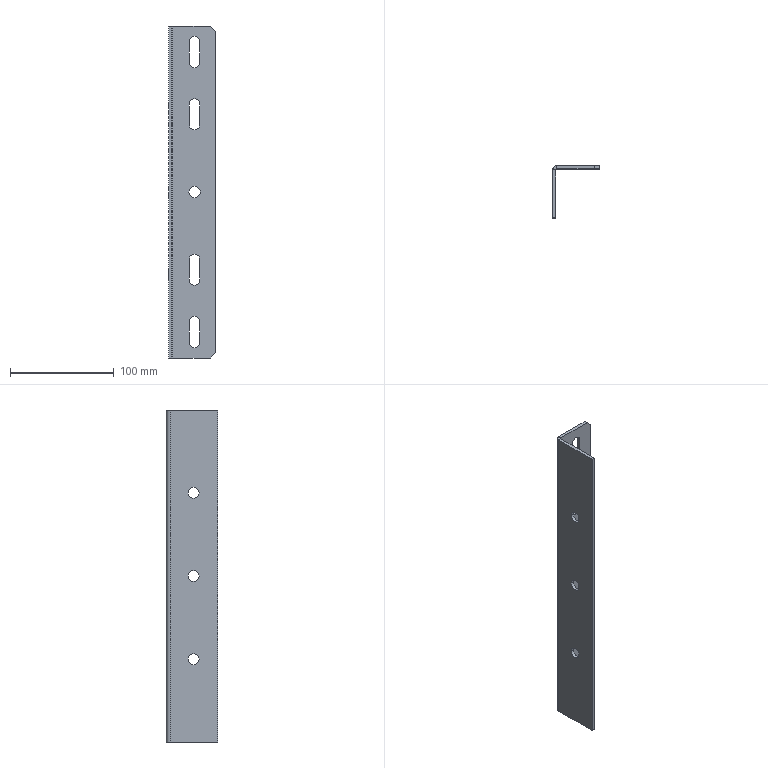Part | SolidWorks | features ICE 3, Chamfer 1, FlatPattern 1, SMBaseFlange 1, SheetMetal 1 | 1 solid | 40 faces | box 45 x 50 x 319.5 mm | volume 82672 mm3 | plane 22 | cylinder 18 | commonest cylinder face diameters 10 x8 10.5 x6 11 x2 2 x1 8 x1
STEP:
#1=CARTESIAN_POINT('',(30.5,0.,0.));
#2=VERTEX_POINT('',#1);
#3=CARTESIAN_POINT('',(19.5,0.,0.));
#4=VERTEX_POINT('',#3);
#5=CARTESIAN_POINT('',(25.,0.,0.));
#6=DIRECTION('',(0.,1.,0.));
#7=DIRECTION('',(1.,0.,0.));
#8=AXIS2_PLACEMENT_3D('',#5,#6,#7);
#9=CIRCLE('',#8,5.5);
#10=EDGE_CURVE('',#2,#4,#9,.T.);
#11=ORIENTED_EDGE('',*,*,#10,.T.);
#12=CARTESIAN_POINT('',(19.5,-3.,0.));
#13=VERTEX_POINT('',#12);
#14=CARTESIAN_POINT('',(19.5,0.000012,0.));
#15=DIRECTION('',(0.,-1.,0.));
#16=VECTOR('',#15,1000.);
#17=LINE('',#14,#16);
#18=EDGE_CURVE('',#4,#13,#17,.T.);
#19=ORIENTED_EDGE('',*,*,#18,.T.);
#20=CARTESIAN_POINT('',(30.5,-3.,0.));
#21=VERTEX_POINT('',#20);
#22=CARTESIAN_POINT('',(25.,-3.,0.));
#23=DIRECTION('',(0.,1.,0.));
#24=DIRECTION('',(1.,0.,0.));
#25=AXIS2_PLACEMENT_3D('',#22,#23,#24);
#26=CIRCLE('',#25,5.5);
#27=EDGE_CURVE('',#21,#13,#26,.T.);
#28=ORIENTED_EDGE('',*,*,#27,.F.);
#29=CARTESIAN_POINT('',(30.5,0.000012,0.));
#30=DIRECTION('',(0.,-1.,0.));
#31=VECTOR('',#30,1000.);
#32=LINE('',#29,#31);
#33=EDGE_CURVE('',#2,#21,#32,.T.);
#34=ORIENTED_EDGE('',*,*,#33,.F.);
#35=EDGE_LOOP('',(#11,#19,#28,#34));
#36=FACE_OUTER_BOUND('',#35,.T.);
#37=CARTESIAN_POINT('',(25.,0.000012,0.));
#38=DIRECTION('',(0.,-1.,0.));
#39=DIRECTION('',(1.,0.,0.));
#40=AXIS2_PLACEMENT_3D('',#37,#38,#39);
#41=CYLINDRICAL_SURFACE('',#40,5.5);
#42=ADVANCED_FACE('',(#36),#41,.F.);
#43=CARTESIAN_POINT('',(3.,-31.75,80.));
#44=VERTEX_POINT('',#43);
#45=CARTESIAN_POINT('',(3.,-21.25,80.));
#46=VERTEX_POINT('',#45);
#47=CARTESIAN_POINT('',(3.,-26.5,80.));
#48=DIRECTION('',(1.,0.,0.));
#49=DIRECTION('',(0.,1.,0.));
#50=AXIS2_PLACEMENT_3D('',#47,#48,#49);
#51=CIRCLE('',#50,5.25);
#52=EDGE_CURVE('',#44,#46,#51,.T.);
#53=ORIENTED_EDGE('',*,*,#52,.T.);
#54=CARTESIAN_POINT('',(0.,-21.25,80.));
#55=VERTEX_POINT('',#54);
#56=CARTESIAN_POINT('',(10.,-21.25,80.));
#57=DIRECTION('',(-1.,0.,0.));
#58=VECTOR('',#57,1000.);
#59=LINE('',#56,#58);
#60=EDGE_CURVE('',#46,#55,#59,.T.);
#61=ORIENTED_EDGE('',*,*,#60,.T.);
#62=CARTESIAN_POINT('',(0.,-31.75,80.));
#63=VERTEX_POINT('',#62);
#64=CARTESIAN_POINT('',(0.,-26.5,80.));
#65=DIRECTION('',(-1.,0.,0.));
#66=DIRECTION('',(0.,-1.,0.));
#67=AXIS2_PLACEMENT_3D('',#64,#65,#66);
#68=CIRCLE('',#67,5.25);
#69=EDGE_CURVE('',#55,#63,#68,.T.);
#70=ORIENTED_EDGE('',*,*,#69,.T.);
#71=CARTESIAN_POINT('',(10.,-31.75,80.));
#72=DIRECTION('',(-1.,0.,0.));
#73=VECTOR('',#72,1000.);
#74=LINE('',#71,#73);
#75=EDGE_CURVE('',#44,#63,#74,.T.);
#76=ORIENTED_EDGE('',*,*,#75,.F.);
#77=EDGE_LOOP('',(#53,#61,#70,#76));
#78=FACE_OUTER_BOUND('',#77,.T.);
#79=CARTESIAN_POINT('',(10.,-26.5,80.));
#80=DIRECTION('',(-1.,0.,0.));
#81=DIRECTION('',(0.,-1.,0.));
#82=AXIS2_PLACEMENT_3D('',#79,#80,#81);
#83=CYLINDRICAL_SURFACE('',#82,5.25);
#84=ADVANCED_FACE('',(#78),#83,.F.);
#85=CARTESIAN_POINT('',(3.,-31.75,0.));
#86=VERTEX_POINT('',#85);
#87=CARTESIAN_POINT('',(3.,-21.25,0.));
#88=VERTEX_POINT('',#87);
#89=CARTESIAN_POINT('',(3.,-26.5,0.));
#90=DIRECTION('',(1.,0.,0.));
#91=DIRECTION('',(0.,1.,0.));
#92=AXIS2_PLACEMENT_3D('',#89,#90,#91);
#93=CIRCLE('',#92,5.25);
#94=EDGE_CURVE('',#86,#88,#93,.T.);
#95=ORIENTED_EDGE('',*,*,#94,.T.);
#96=CARTESIAN_POINT('',(0.,-21.25,0.));
#97=VERTEX_POINT('',#96);
#98=CARTESIAN_POINT('',(10.,-21.25,0.));
#99=DIRECTION('',(-1.,0.,0.));
#100=VECTOR('',#99,1000.);
#101=LINE('',#98,#100);
#102=EDGE_CURVE('',#88,#97,#101,.T.);
#103=ORIENTED_EDGE('',*,*,#102,.T.);
#104=CARTESIAN_POINT('',(0.,-31.75,0.));
#105=VERTEX_POINT('',#104);
#106=CARTESIAN_POINT('',(0.,-26.5,0.));
#107=DIRECTION('',(-1.,0.,0.));
#108=DIRECTION('',(0.,-1.,0.));
#109=AXIS2_PLACEMENT_3D('',#106,#107,#108);
#110=CIRCLE('',#109,5.25);
#111=EDGE_CURVE('',#97,#105,#110,.T.);
#112=ORIENTED_EDGE('',*,*,#111,.T.);
#113=CARTESIAN_POINT('',(10.,-31.75,0.));
#114=DIRECTION('',(-1.,0.,0.));
#115=VECTOR('',#114,1000.);
#116=LINE('',#113,#115);
#117=EDGE_CURVE('',#86,#105,#116,.T.);
#118=ORIENTED_EDGE('',*,*,#117,.F.);
#119=EDGE_LOOP('',(#95,#103,#112,#118));
#120=FACE_OUTER_BOUND('',#119,.T.);
#121=CARTESIAN_POINT('',(10.,-26.5,0.));
#122=DIRECTION('',(-1.,0.,0.));
#123=DIRECTION('',(0.,-1.,0.));
#124=AXIS2_PLACEMENT_3D('',#121,#122,#123);
#125=CYLINDRICAL_SURFACE('',#124,5.25);
#126=ADVANCED_FACE('',(#120),#125,.F.);
#127=CARTESIAN_POINT('',(3.,-31.75,-80.));
#128=VERTEX_POINT('',#127);
#129=CARTESIAN_POINT('',(3.,-21.25,-80.));
#130=VERTEX_POINT('',#129);
#131=CARTESIAN_POINT('',(3.,-26.5,-80.));
#132=DIRECTION('',(1.,0.,0.));
#133=DIRECTION('',(0.,1.,0.));
#134=AXIS2_PLACEMENT_3D('',#131,#132,#133);
#135=CIRCLE('',#134,5.25);
#136=EDGE_CURVE('',#128,#130,#135,.T.);
#137=ORIENTED_EDGE('',*,*,#136,.T.);
#138=CARTESIAN_POINT('',(0.,-21.25,-80.));
#139=VERTEX_POINT('',#138);
#140=CARTESIAN_POINT('',(10.,-21.25,-80.));
#141=DIRECTION('',(-1.,0.,0.));
#142=VECTOR('',#141,1000.);
#143=LINE('',#140,#142);
#144=EDGE_CURVE('',#130,#139,#143,.T.);
#145=ORIENTED_EDGE('',*,*,#144,.T.);
#146=CARTESIAN_POINT('',(0.,-31.75,-80.));
#147=VERTEX_POINT('',#146);
#148=CARTESIAN_POINT('',(0.,-26.5,-80.));
#149=DIRECTION('',(-1.,0.,0.));
#150=DIRECTION('',(0.,-1.,0.));
#151=AXIS2_PLACEMENT_3D('',#148,#149,#150);
#152=CIRCLE('',#151,5.25);
#153=EDGE_CURVE('',#139,#147,#152,.T.);
#154=ORIENTED_EDGE('',*,*,#153,.T.);
#155=CARTESIAN_POINT('',(10.,-31.75,-80.));
#156=DIRECTION('',(-1.,0.,0.));
#157=VECTOR('',#156,1000.);
#158=LINE('',#155,#157);
#159=EDGE_CURVE('',#128,#147,#158,.T.);
#160=ORIENTED_EDGE('',*,*,#159,.F.);
#161=EDGE_LOOP('',(#137,#145,#154,#160));
#162=FACE_OUTER_BOUND('',#161,.T.);
#163=CARTESIAN_POINT('',(10.,-26.5,-80.));
#164=DIRECTION('',(-1.,0.,0.));
#165=DIRECTION('',(0.,-1.,0.));
#166=AXIS2_PLACEMENT_3D('',#163,#164,#165);
#167=CYLINDRICAL_SURFACE('',#166,5.25);
#168=ADVANCED_FACE('',(#162),#167,.F.);
#169=CARTESIAN_POINT('',(4.,0.,159.75));
#170=VERTEX_POINT('',#169);
#171=CARTESIAN_POINT('',(4.,-3.,159.75));
#172=VERTEX_POINT('',#171);
#173=CARTESIAN_POINT('',(4.,0.,159.75));
#174=DIRECTION('',(0.,-1.,0.));
#175=VECTOR('',#174,1000.);
#176=LINE('',#173,#175);
#177=EDGE_CURVE('',#170,#172,#176,.T.);
#178=ORIENTED_EDGE('',*,*,#177,.F.);
#179=CARTESIAN_POINT('',(0.,-4.,159.75));
#180=VERTEX_POINT('',#179);
#181=CARTESIAN_POINT('',(4.,-4.,159.75));
#182=DIRECTION('',(0.,0.,1.));
#183=DIRECTION('',(-1.,0.,0.));
#184=AXIS2_PLACEMENT_3D('',#181,#182,#183);
#185=CIRCLE('',#184,4.);
#186=EDGE_CURVE('',#170,#180,#185,.T.);
#187=ORIENTED_EDGE('',*,*,#186,.T.);
#188=CARTESIAN_POINT('',(3.,-4.,159.75));
#189=VERTEX_POINT('',#188);
#190=CARTESIAN_POINT('',(3.,-4.,159.75));
#191=DIRECTION('',(-1.,0.,0.));
#192=VECTOR('',#191,1000.);
#193=LINE('',#190,#192);
#194=EDGE_CURVE('',#189,#180,#193,.T.);
#195=ORIENTED_EDGE('',*,*,#194,.F.);
#196=CARTESIAN_POINT('',(4.,-4.,159.75));
#197=DIRECTION('',(0.,0.,1.));
#198=DIRECTION('',(1.,0.,0.));
#199=AXIS2_PLACEMENT_3D('',#196,#197,#198);
#200=CIRCLE('',#199,1.);
#201=EDGE_CURVE('',#172,#189,#200,.T.);
#202=ORIENTED_EDGE('',*,*,#201,.F.);
#203=EDGE_LOOP('',(#178,#187,#195,#202));
#204=FACE_OUTER_BOUND('',#203,.T.);
#205=CARTESIAN_POINT('',(4.,0.,159.75));
#206=DIRECTION('',(0.,0.,1.));
#207=DIRECTION('',(1.,0.,0.));
#208=AXIS2_PLACEMENT_3D('',#205,#206,#207);
#209=PLANE('',#208);
#210=ADVANCED_FACE('',(#204),#209,.T.);
#211=CARTESIAN_POINT('',(40.,-3.,159.75));
#212=VERTEX_POINT('',#211);
#213=CARTESIAN_POINT('',(45.,-3.,159.75));
#214=DIRECTION('',(-1.,0.,0.));
#215=VECTOR('',#214,1000.);
#216=LINE('',#213,#215);
#217=EDGE_CURVE('',#212,#172,#216,.T.);
#218=ORIENTED_EDGE('',*,*,#217,.F.);
#219=CARTESIAN_POINT('',(40.,0.,159.75));
#220=VERTEX_POINT('',#219);
#221=CARTESIAN_POINT('',(40.,-4.,159.75));
#222=DIRECTION('',(0.,1.,0.));
#223=VECTOR('',#222,1000.);
#224=LINE('',#221,#223);
#225=EDGE_CURVE('',#212,#220,#224,.T.);
#226=ORIENTED_EDGE('',*,*,#225,.T.);
#227=CARTESIAN_POINT('',(45.,0.,159.75));
#228=DIRECTION('',(-1.,0.,0.));
#229=VECTOR('',#228,1000.);
#230=LINE('',#227,#229);
#231=EDGE_CURVE('',#220,#170,#230,.T.);
#232=ORIENTED_EDGE('',*,*,#231,.T.);
#233=ORIENTED_EDGE('',*,*,#177,.T.);
#234=EDGE_LOOP('',(#218,#226,#232,#233));
#235=FACE_OUTER_BOUND('',#234,.T.);
#236=CARTESIAN_POINT('',(3.,-4.,159.75));
#237=DIRECTION('',(0.,0.,1.));
#238=DIRECTION('',(1.,0.,0.));
#239=AXIS2_PLACEMENT_3D('',#236,#237,#238);
#240=PLANE('',#239);
#241=ADVANCED_FACE('',(#235),#240,.T.);
#242=CARTESIAN_POINT('',(0.,-4.,-159.75));
#243=VERTEX_POINT('',#242);
#244=CARTESIAN_POINT('',(3.,-4.,-159.75));
#245=VERTEX_POINT('',#244);
#246=CARTESIAN_POINT('',(0.,-4.,-159.75));
#247=DIRECTION('',(1.,0.,0.));
#248=VECTOR('',#247,1000.);
#249=LINE('',#246,#248);
#250=EDGE_CURVE('',#243,#245,#249,.T.);
#251=ORIENTED_EDGE('',*,*,#250,.F.);
#252=CARTESIAN_POINT('',(4.,0.,-159.75));
#253=VERTEX_POINT('',#252);
#254=CARTESIAN_POINT('',(4.,-4.,-159.75));
#255=DIRECTION('',(0.,0.,1.));
#256=DIRECTION('',(-1.,0.,0.));
#257=AXIS2_PLACEMENT_3D('',#254,#255,#256);
#258=CIRCLE('',#257,4.);
#259=EDGE_CURVE('',#253,#243,#258,.T.);
#260=ORIENTED_EDGE('',*,*,#259,.F.);
#261=CARTESIAN_POINT('',(4.,-3.,-159.75));
#262=VERTEX_POINT('',#261);
#263=CARTESIAN_POINT('',(4.,-3.,-159.75));
#264=DIRECTION('',(0.,1.,0.));
#265=VECTOR('',#264,1000.);
#266=LINE('',#263,#265);
#267=EDGE_CURVE('',#262,#253,#266,.T.);
#268=ORIENTED_EDGE('',*,*,#267,.F.);
#269=CARTESIAN_POINT('',(4.,-4.,-159.75));
#270=DIRECTION('',(0.,0.,1.));
#271=DIRECTION('',(1.,0.,0.));
#272=AXIS2_PLACEMENT_3D('',#269,#270,#271);
#273=CIRCLE('',#272,1.);
#274=EDGE_CURVE('',#262,#245,#273,.T.);
#275=ORIENTED_EDGE('',*,*,#274,.T.);
#276=EDGE_LOOP('',(#251,#260,#268,#275));
#277=FACE_OUTER_BOUND('',#276,.T.);
#278=CARTESIAN_POINT('',(0.,-4.,-159.75));
#279=DIRECTION('',(0.,0.,-1.));
#280=DIRECTION('',(-1.,0.,0.));
#281=AXIS2_PLACEMENT_3D('',#278,#279,#280);
#282=PLANE('',#281);
#283=ADVANCED_FACE('',(#277),#282,.T.);
#284=CARTESIAN_POINT('',(0.,-50.,-159.75));
#285=VERTEX_POINT('',#284);
#286=CARTESIAN_POINT('',(0.,0.,-159.75));
#287=DIRECTION('',(0.,-1.,0.));
#288=VECTOR('',#287,1000.);
#289=LINE('',#286,#288);
#290=EDGE_CURVE('',#243,#285,#289,.T.);
#291=ORIENTED_EDGE('',*,*,#290,.F.);
#292=ORIENTED_EDGE('',*,*,#250,.T.);
#293=CARTESIAN_POINT('',(3.,-50.,-159.75));
#294=VERTEX_POINT('',#293);
#295=CARTESIAN_POINT('',(3.,0.,-159.75));
#296=DIRECTION('',(0.,-1.,0.));
#297=VECTOR('',#296,1000.);
#298=LINE('',#295,#297);
#299=EDGE_CURVE('',#245,#294,#298,.T.);
#300=ORIENTED_EDGE('',*,*,#299,.T.);
#301=CARTESIAN_POINT('',(3.,-50.,-159.75));
#302=DIRECTION('',(-1.,0.,0.));
#303=VECTOR('',#302,1000.);
#304=LINE('',#301,#303);
#305=EDGE_CURVE('',#294,#285,#304,.T.);
#306=ORIENTED_EDGE('',*,*,#305,.T.);
#307=EDGE_LOOP('',(#291,#292,#300,#306));
#308=FACE_OUTER_BOUND('',#307,.T.);
#309=CARTESIAN_POINT('',(4.,-3.,-159.75));
#310=DIRECTION('',(0.,0.,-1.));
#311=DIRECTION('',(-1.,0.,0.));
#312=AXIS2_PLACEMENT_3D('',#309,#310,#311);
#313=PLANE('',#312);
#314=ADVANCED_FACE('',(#308),#313,.T.);
#315=CARTESIAN_POINT('',(0.,-26.5,80.));
#316=DIRECTION('',(-1.,0.,0.));
#317=DIRECTION('',(0.,-1.,0.));
#318=AXIS2_PLACEMENT_3D('',#315,#316,#317);
#319=CIRCLE('',#318,5.25);
#320=EDGE_CURVE('',#63,#55,#319,.T.);
#321=ORIENTED_EDGE('',*,*,#320,.F.);
#322=ORIENTED_EDGE('',*,*,#69,.F.);
#323=EDGE_LOOP('',(#321,#322));
#324=FACE_BOUND('',#323,.T.);
#325=CARTESIAN_POINT('',(0.,-26.5,0.));
#326=DIRECTION('',(-1.,0.,0.));
#327=DIRECTION('',(0.,-1.,0.));
#328=AXIS2_PLACEMENT_3D('',#325,#326,#327);
#329=CIRCLE('',#328,5.25);
#330=EDGE_CURVE('',#105,#97,#329,.T.);
#331=ORIENTED_EDGE('',*,*,#330,.F.);
#332=ORIENTED_EDGE('',*,*,#111,.F.);
#333=EDGE_LOOP('',(#331,#332));
#334=FACE_BOUND('',#333,.T.);
#335=CARTESIAN_POINT('',(0.,-26.5,-80.));
#336=DIRECTION('',(-1.,0.,0.));
#337=DIRECTION('',(0.,-1.,0.));
#338=AXIS2_PLACEMENT_3D('',#335,#336,#337);
#339=CIRCLE('',#338,5.25);
#340=EDGE_CURVE('',#147,#139,#339,.T.);
#341=ORIENTED_EDGE('',*,*,#340,.F.);
#342=ORIENTED_EDGE('',*,*,#153,.F.);
#343=EDGE_LOOP('',(#341,#342));
#344=FACE_BOUND('',#343,.T.);
#345=ORIENTED_EDGE('',*,*,#290,.T.);
#346=CARTESIAN_POINT('',(0.,-50.,159.75));
#347=VERTEX_POINT('',#346);
#348=CARTESIAN_POINT('',(0.,-50.,159.75));
#349=DIRECTION('',(0.,0.,-1.));
#350=VECTOR('',#349,1000.);
#351=LINE('',#348,#350);
#352=EDGE_CURVE('',#347,#285,#351,.T.);
#353=ORIENTED_EDGE('',*,*,#352,.F.);
#354=CARTESIAN_POINT('',(0.,0.,159.75));
#355=DIRECTION('',(0.,-1.,0.));
#356=VECTOR('',#355,1000.);
#357=LINE('',#354,#356);
#358=EDGE_CURVE('',#180,#347,#357,.T.);
#359=ORIENTED_EDGE('',*,*,#358,.F.);
#360=CARTESIAN_POINT('',(0.,-4.,159.75));
#361=DIRECTION('',(0.,0.,-1.));
#362=VECTOR('',#361,1000.);
#363=LINE('',#360,#362);
#364=EDGE_CURVE('',#180,#243,#363,.T.);
#365=ORIENTED_EDGE('',*,*,#364,.T.);
#366=EDGE_LOOP('',(#345,#353,#359,#365));
#367=FACE_OUTER_BOUND('',#366,.T.);
#368=CARTESIAN_POINT('',(0.,0.,159.75));
#369=DIRECTION('',(1.,0.,0.));
#370=DIRECTION('',(0.,1.,0.));
#371=AXIS2_PLACEMENT_3D('',#368,#369,#370);
#372=PLANE('',#371);
#373=ADVANCED_FACE('',(#324,#334,#344,#367),#372,.F.);
#374=ORIENTED_EDGE('',*,*,#305,.F.);
#375=CARTESIAN_POINT('',(3.,-50.,159.75));
#376=VERTEX_POINT('',#375);
#377=CARTESIAN_POINT('',(3.,-50.,159.75));
#378=DIRECTION('',(0.,0.,-1.));
#379=VECTOR('',#378,1000.);
#380=LINE('',#377,#379);
#381=EDGE_CURVE('',#376,#294,#380,.T.);
#382=ORIENTED_EDGE('',*,*,#381,.F.);
#383=CARTESIAN_POINT('',(3.,-50.,159.75));
#384=DIRECTION('',(-1.,0.,0.));
#385=VECTOR('',#384,1000.);
#386=LINE('',#383,#385);
#387=EDGE_CURVE('',#376,#347,#386,.T.);
#388=ORIENTED_EDGE('',*,*,#387,.T.);
#389=ORIENTED_EDGE('',*,*,#352,.T.);
#390=EDGE_LOOP('',(#374,#382,#388,#389));
#391=FACE_OUTER_BOUND('',#390,.T.);
#392=CARTESIAN_POINT('',(3.,-50.,159.75));
#393=DIRECTION('',(0.,-1.,0.));
#394=DIRECTION('',(0.,0.,-1.));
#395=AXIS2_PLACEMENT_3D('',#392,#393,#394);
#396=PLANE('',#395);
#397=ADVANCED_FACE('',(#391),#396,.T.);
#398=ORIENTED_EDGE('',*,*,#52,.F.);
#399=CARTESIAN_POINT('',(3.,-26.5,80.));
#400=DIRECTION('',(1.,0.,0.));
#401=DIRECTION('',(0.,1.,0.));
#402=AXIS2_PLACEMENT_3D('',#399,#400,#401);
#403=CIRCLE('',#402,5.25);
#404=EDGE_CURVE('',#46,#44,#403,.T.);
#405=ORIENTED_EDGE('',*,*,#404,.F.);
#406=EDGE_LOOP('',(#398,#405));
#407=FACE_BOUND('',#406,.T.);
#408=ORIENTED_EDGE('',*,*,#94,.F.);
#409=CARTESIAN_POINT('',(3.,-26.5,0.));
#410=DIRECTION('',(1.,0.,0.));
#411=DIRECTION('',(0.,1.,0.));
#412=AXIS2_PLACEMENT_3D('',#409,#410,#411);
#413=CIRCLE('',#412,5.25);
#414=EDGE_CURVE('',#88,#86,#413,.T.);
#415=ORIENTED_EDGE('',*,*,#414,.F.);
#416=EDGE_LOOP('',(#408,#415));
#417=FACE_BOUND('',#416,.T.);
#418=ORIENTED_EDGE('',*,*,#136,.F.);
#419=CARTESIAN_POINT('',(3.,-26.5,-80.));
#420=DIRECTION('',(1.,0.,0.));
#421=DIRECTION('',(0.,1.,0.));
#422=AXIS2_PLACEMENT_3D('',#419,#420,#421);
#423=CIRCLE('',#422,5.25);
#424=EDGE_CURVE('',#130,#128,#423,.T.);
#425=ORIENTED_EDGE('',*,*,#424,.F.);
#426=EDGE_LOOP('',(#418,#425));
#427=FACE_BOUND('',#426,.T.);
#428=ORIENTED_EDGE('',*,*,#299,.F.);
#429=CARTESIAN_POINT('',(3.,-4.,159.75));
#430=DIRECTION('',(0.,0.,-1.));
#431=VECTOR('',#430,1000.);
#432=LINE('',#429,#431);
#433=EDGE_CURVE('',#189,#245,#432,.T.);
#434=ORIENTED_EDGE('',*,*,#433,.F.);
#435=CARTESIAN_POINT('',(3.,0.,159.75));
#436=DIRECTION('',(0.,-1.,0.));
#437=VECTOR('',#436,1000.);
#438=LINE('',#435,#437);
#439=EDGE_CURVE('',#189,#376,#438,.T.);
#440=ORIENTED_EDGE('',*,*,#439,.T.);
#441=ORIENTED_EDGE('',*,*,#381,.T.);
#442=EDGE_LOOP('',(#428,#434,#440,#441));
#443=FACE_OUTER_BOUND('',#442,.T.);
#444=CARTESIAN_POINT('',(3.,0.,159.75));
#445=DIRECTION('',(1.,0.,0.));
#446=DIRECTION('',(0.,1.,0.));
#447=AXIS2_PLACEMENT_3D('',#444,#445,#446);
#448=PLANE('',#447);
#449=ADVANCED_FACE('',(#407,#417,#427,#443),#448,.T.);
#450=ORIENTED_EDGE('',*,*,#274,.F.);
#451=CARTESIAN_POINT('',(4.,-3.,159.75));
#452=DIRECTION('',(0.,0.,-1.));
#453=VECTOR('',#452,1000.);
#454=LINE('',#451,#453);
#455=EDGE_CURVE('',#172,#262,#454,.T.);
#456=ORIENTED_EDGE('',*,*,#455,.F.);
#457=ORIENTED_EDGE('',*,*,#201,.T.);
#458=ORIENTED_EDGE('',*,*,#433,.T.);
#459=EDGE_LOOP('',(#450,#456,#457,#458));
#460=FACE_OUTER_BOUND('',#459,.T.);
#461=CARTESIAN_POINT('',(4.,-4.,159.75));
#462=DIRECTION('',(0.,0.,-1.));
#463=DIRECTION('',(-1.,0.,0.));
#464=AXIS2_PLACEMENT_3D('',#461,#462,#463);
#465=CYLINDRICAL_SURFACE('',#464,1.);
#466=ADVANCED_FACE('',(#460),#465,.F.);
#467=ORIENTED_EDGE('',*,*,#27,.T.);
#468=CARTESIAN_POINT('',(25.,-3.,0.));
#469=DIRECTION('',(0.,1.,0.));
#470=DIRECTION('',(1.,0.,0.));
#471=AXIS2_PLACEMENT_3D('',#468,#469,#470);
#472=CIRCLE('',#471,5.5);
#473=EDGE_CURVE('',#13,#21,#472,.T.);
#474=ORIENTED_EDGE('',*,*,#473,.T.);
#475=EDGE_LOOP('',(#467,#474));
#476=FACE_BOUND('',#475,.T.);
#477=CARTESIAN_POINT('',(30.,-3.,144.75));
#478=VERTEX_POINT('',#477);
#479=CARTESIAN_POINT('',(20.,-3.,144.75));
#480=VERTEX_POINT('',#479);
#481=CARTESIAN_POINT('',(25.,-3.,144.75));
#482=DIRECTION('',(0.,-1.,0.));
#483=DIRECTION('',(1.,0.,0.));
#484=AXIS2_PLACEMENT_3D('',#481,#482,#483);
#485=CIRCLE('',#484,5.);
#486=EDGE_CURVE('',#478,#480,#485,.T.);
#487=ORIENTED_EDGE('',*,*,#486,.F.);
#488=CARTESIAN_POINT('',(30.,-3.,124.75));
#489=VERTEX_POINT('',#488);
#490=CARTESIAN_POINT('',(30.,-3.,159.75));
#491=DIRECTION('',(0.,0.,1.));
#492=VECTOR('',#491,1000.);
#493=LINE('',#490,#492);
#494=EDGE_CURVE('',#489,#478,#493,.T.);
#495=ORIENTED_EDGE('',*,*,#494,.F.);
#496=CARTESIAN_POINT('',(20.,-3.,124.75));
#497=VERTEX_POINT('',#496);
#498=CARTESIAN_POINT('',(25.,-3.,124.75));
#499=DIRECTION('',(0.,-1.,0.));
#500=DIRECTION('',(1.,0.,0.));
#501=AXIS2_PLACEMENT_3D('',#498,#499,#500);
#502=CIRCLE('',#501,5.);
#503=EDGE_CURVE('',#497,#489,#502,.T.);
#504=ORIENTED_EDGE('',*,*,#503,.F.);
#505=CARTESIAN_POINT('',(20.,-3.,159.75));
#506=DIRECTION('',(0.,0.,-1.));
#507=VECTOR('',#506,1000.);
#508=LINE('',#505,#507);
#509=EDGE_CURVE('',#480,#497,#508,.T.);
#510=ORIENTED_EDGE('',*,*,#509,.F.);
#511=EDGE_LOOP('',(#487,#495,#504,#510));
#512=FACE_BOUND('',#511,.T.);
#513=CARTESIAN_POINT('',(20.,-3.,-84.75));
#514=VERTEX_POINT('',#513);
#515=CARTESIAN_POINT('',(30.,-3.,-84.75));
#516=VERTEX_POINT('',#515);
#517=CARTESIAN_POINT('',(25.,-3.,-84.75));
#518=DIRECTION('',(0.,-1.,0.));
#519=DIRECTION('',(1.,0.,0.));
#520=AXIS2_PLACEMENT_3D('',#517,#518,#519);
#521=CIRCLE('',#520,5.);
#522=EDGE_CURVE('',#514,#516,#521,.T.);
#523=ORIENTED_EDGE('',*,*,#522,.F.);
#524=CARTESIAN_POINT('',(20.,-3.,-64.75));
#525=VERTEX_POINT('',#524);
#526=CARTESIAN_POINT('',(20.,-3.,159.75));
#527=DIRECTION('',(0.,0.,-1.));
#528=VECTOR('',#527,1000.);
#529=LINE('',#526,#528);
#530=EDGE_CURVE('',#525,#514,#529,.T.);
#531=ORIENTED_EDGE('',*,*,#530,.F.);
#532=CARTESIAN_POINT('',(30.,-3.,-64.75));
#533=VERTEX_POINT('',#532);
#534=CARTESIAN_POINT('',(25.,-3.,-64.75));
#535=DIRECTION('',(0.,-1.,0.));
#536=DIRECTION('',(1.,0.,0.));
#537=AXIS2_PLACEMENT_3D('',#534,#535,#536);
#538=CIRCLE('',#537,5.);
#539=EDGE_CURVE('',#533,#525,#538,.T.);
#540=ORIENTED_EDGE('',*,*,#539,.F.);
#541=CARTESIAN_POINT('',(30.,-3.,159.75));
#542=DIRECTION('',(0.,0.,1.));
#543=VECTOR('',#542,1000.);
#544=LINE('',#541,#543);
#545=EDGE_CURVE('',#516,#533,#544,.T.);
#546=ORIENTED_EDGE('',*,*,#545,.F.);
#547=EDGE_LOOP('',(#523,#531,#540,#546));
#548=FACE_BOUND('',#547,.T.);
#549=CARTESIAN_POINT('',(20.,-3.,-144.75));
#550=VERTEX_POINT('',#549);
#551=CARTESIAN_POINT('',(30.,-3.,-144.75));
#552=VERTEX_POINT('',#551);
#553=CARTESIAN_POINT('',(25.,-3.,-144.75));
#554=DIRECTION('',(0.,-1.,0.));
#555=DIRECTION('',(1.,0.,0.));
#556=AXIS2_PLACEMENT_3D('',#553,#554,#555);
#557=CIRCLE('',#556,5.);
#558=EDGE_CURVE('',#550,#552,#557,.T.);
#559=ORIENTED_EDGE('',*,*,#558,.F.);
#560=CARTESIAN_POINT('',(20.,-3.,-124.75));
#561=VERTEX_POINT('',#560);
#562=CARTESIAN_POINT('',(20.,-3.,159.75));
#563=DIRECTION('',(0.,0.,-1.));
#564=VECTOR('',#563,1000.);
#565=LINE('',#562,#564);
#566=EDGE_CURVE('',#561,#550,#565,.T.);
#567=ORIENTED_EDGE('',*,*,#566,.F.);
#568=CARTESIAN_POINT('',(30.,-3.,-124.75));
#569=VERTEX_POINT('',#568);
#570=CARTESIAN_POINT('',(25.,-3.,-124.75));
#571=DIRECTION('',(0.,-1.,0.));
#572=DIRECTION('',(1.,0.,0.));
#573=AXIS2_PLACEMENT_3D('',#570,#571,#572);
#574=CIRCLE('',#573,5.);
#575=EDGE_CURVE('',#569,#561,#574,.T.);
#576=ORIENTED_EDGE('',*,*,#575,.F.);
#577=CARTESIAN_POINT('',(30.,-3.,159.75));
#578=DIRECTION('',(0.,0.,1.));
#579=VECTOR('',#578,1000.);
#580=LINE('',#577,#579);
#581=EDGE_CURVE('',#552,#569,#580,.T.);
#582=ORIENTED_EDGE('',*,*,#581,.F.);
#583=EDGE_LOOP('',(#559,#567,#576,#582));
#584=FACE_BOUND('',#583,.T.);
#585=CARTESIAN_POINT('',(30.,-3.,84.75));
#586=VERTEX_POINT('',#585);
#587=CARTESIAN_POINT('',(20.,-3.,84.75));
#588=VERTEX_POINT('',#587);
#589=CARTESIAN_POINT('',(25.,-3.,84.75));
#590=DIRECTION('',(0.,-1.,0.));
#591=DIRECTION('',(1.,0.,0.));
#592=AXIS2_PLACEMENT_3D('',#589,#590,#591);
#593=CIRCLE('',#592,5.);
#594=EDGE_CURVE('',#586,#588,#593,.T.);
#595=ORIENTED_EDGE('',*,*,#594,.F.);
#596=CARTESIAN_POINT('',(30.,-3.,64.75));
#597=VERTEX_POINT('',#596);
#598=CARTESIAN_POINT('',(30.,-3.,159.75));
#599=DIRECTION('',(0.,0.,1.));
#600=VECTOR('',#599,1000.);
#601=LINE('',#598,#600);
#602=EDGE_CURVE('',#597,#586,#601,.T.);
#603=ORIENTED_EDGE('',*,*,#602,.F.);
#604=CARTESIAN_POINT('',(20.,-3.,64.75));
#605=VERTEX_POINT('',#604);
#606=CARTESIAN_POINT('',(25.,-3.,64.75));
#607=DIRECTION('',(0.,-1.,0.));
#608=DIRECTION('',(1.,0.,0.));
#609=AXIS2_PLACEMENT_3D('',#606,#607,#608);
#610=CIRCLE('',#609,5.);
#611=EDGE_CURVE('',#605,#597,#610,.T.);
#612=ORIENTED_EDGE('',*,*,#611,.F.);
#613=CARTESIAN_POINT('',(20.,-3.,159.75));
#614=DIRECTION('',(0.,0.,-1.));
#615=VECTOR('',#614,1000.);
#616=LINE('',#613,#615);
#617=EDGE_CURVE('',#588,#605,#616,.T.);
#618=ORIENTED_EDGE('',*,*,#617,.F.);
#619=EDGE_LOOP('',(#595,#603,#612,#618));
#620=FACE_BOUND('',#619,.T.);
#621=CARTESIAN_POINT('',(40.,-3.,-159.75));
#622=VERTEX_POINT('',#621);
#623=CARTESIAN_POINT('',(45.,-3.,-159.75));
#624=DIRECTION('',(-1.,0.,0.));
#625=VECTOR('',#624,1000.);
#626=LINE('',#623,#625);
#627=EDGE_CURVE('',#622,#262,#626,.T.);
#628=ORIENTED_EDGE('',*,*,#627,.F.);
#629=CARTESIAN_POINT('',(45.,-3.,-154.75));
#630=VERTEX_POINT('',#629);
#631=CARTESIAN_POINT('',(202.25,-3.,2.5));
#632=DIRECTION('',(0.7071,0.,0.7071));
#633=VECTOR('',#632,1000.);
#634=LINE('',#631,#633);
#635=EDGE_CURVE('',#622,#630,#634,.T.);
#636=ORIENTED_EDGE('',*,*,#635,.T.);
#637=CARTESIAN_POINT('',(45.,-3.,154.75));
#638=VERTEX_POINT('',#637);
#639=CARTESIAN_POINT('',(45.,-3.,159.75));
#640=DIRECTION('',(0.,0.,-1.));
#641=VECTOR('',#640,1000.);
#642=LINE('',#639,#641);
#643=EDGE_CURVE('',#638,#630,#642,.T.);
#644=ORIENTED_EDGE('',*,*,#643,.F.);
#645=CARTESIAN_POINT('',(42.5,-3.,157.25));
#646=DIRECTION('',(-0.7071,0.,0.7071));
#647=VECTOR('',#646,1000.);
#648=LINE('',#645,#647);
#649=EDGE_CURVE('',#638,#212,#648,.T.);
#650=ORIENTED_EDGE('',*,*,#649,.T.);
#651=ORIENTED_EDGE('',*,*,#217,.T.);
#652=ORIENTED_EDGE('',*,*,#455,.T.);
#653=EDGE_LOOP('',(#628,#636,#644,#650,#651,#652));
#654=FACE_OUTER_BOUND('',#653,.T.);
#655=CARTESIAN_POINT('',(45.,-3.,159.75));
#656=DIRECTION('',(0.,-1.,0.));
#657=DIRECTION('',(1.,0.,0.));
#658=AXIS2_PLACEMENT_3D('',#655,#656,#657);
#659=PLANE('',#658);
#660=ADVANCED_FACE('',(#476,#512,#548,#584,#620,#654),#659,.T.);
#661=ORIENTED_EDGE('',*,*,#643,.T.);
#662=CARTESIAN_POINT('',(45.,0.,-154.75));
#663=VERTEX_POINT('',#662);
#664=CARTESIAN_POINT('',(45.,0.,-154.75));
#665=DIRECTION('',(0.,1.,0.));
#666=VECTOR('',#665,1000.);
#667=LINE('',#664,#666);
#668=EDGE_CURVE('',#630,#663,#667,.T.);
#669=ORIENTED_EDGE('',*,*,#668,.T.);
#670=CARTESIAN_POINT('',(45.,0.,154.75));
#671=VERTEX_POINT('',#670);
#672=CARTESIAN_POINT('',(45.,0.,159.75));
#673=DIRECTION('',(0.,0.,-1.));
#674=VECTOR('',#673,1000.);
#675=LINE('',#672,#674);
#676=EDGE_CURVE('',#671,#663,#675,.T.);
#677=ORIENTED_EDGE('',*,*,#676,.F.);
#678=CARTESIAN_POINT('',(45.,0.,154.75));
#679=DIRECTION('',(0.,-1.,0.));
#680=VECTOR('',#679,1000.);
#681=LINE('',#678,#680);
#682=EDGE_CURVE('',#671,#638,#681,.T.);
#683=ORIENTED_EDGE('',*,*,#682,.T.);
#684=EDGE_LOOP('',(#661,#669,#677,#683));
#685=FACE_OUTER_BOUND('',#684,.T.);
#686=CARTESIAN_POINT('',(45.,0.,159.75));
#687=DIRECTION('',(1.,0.,0.));
#688=DIRECTION('',(0.,0.,-1.));
#689=AXIS2_PLACEMENT_3D('',#686,#687,#688);
#690=PLANE('',#689);
#691=ADVANCED_FACE('',(#685),#690,.T.);
#692=ORIENTED_EDGE('',*,*,#10,.F.);
#693=CARTESIAN_POINT('',(25.,0.,0.));
#694=DIRECTION('',(0.,1.,0.));
#695=DIRECTION('',(1.,0.,0.));
#696=AXIS2_PLACEMENT_3D('',#693,#694,#695);
#697=CIRCLE('',#696,5.5);
#698=EDGE_CURVE('',#4,#2,#697,.T.);
#699=ORIENTED_EDGE('',*,*,#698,.F.);
#700=EDGE_LOOP('',(#692,#699));
#701=FACE_BOUND('',#700,.T.);
#702=CARTESIAN_POINT('',(30.,0.,144.75));
#703=VERTEX_POINT('',#702);
#704=CARTESIAN_POINT('',(30.,0.,124.75));
#705=VERTEX_POINT('',#704);
#706=CARTESIAN_POINT('',(30.,0.,144.75));
#707=DIRECTION('',(0.,0.,-1.));
#708=VECTOR('',#707,1000.);
#709=LINE('',#706,#708);
#710=EDGE_CURVE('',#703,#705,#709,.T.);
#711=ORIENTED_EDGE('',*,*,#710,.F.);
#712=CARTESIAN_POINT('',(20.,0.,144.75));
#713=VERTEX_POINT('',#712);
#714=CARTESIAN_POINT('',(25.,0.,144.75));
#715=DIRECTION('',(0.,1.,0.));
#716=DIRECTION('',(1.,0.,0.));
#717=AXIS2_PLACEMENT_3D('',#714,#715,#716);
#718=CIRCLE('',#717,5.);
#719=EDGE_CURVE('',#713,#703,#718,.T.);
#720=ORIENTED_EDGE('',*,*,#719,.F.);
#721=CARTESIAN_POINT('',(20.,0.,124.75));
#722=VERTEX_POINT('',#721);
#723=CARTESIAN_POINT('',(20.,0.,144.75));
#724=DIRECTION('',(0.,0.,1.));
#725=VECTOR('',#724,1000.);
#726=LINE('',#723,#725);
#727=EDGE_CURVE('',#722,#713,#726,.T.);
#728=ORIENTED_EDGE('',*,*,#727,.F.);
#729=CARTESIAN_POINT('',(25.,0.,124.75));
#730=DIRECTION('',(0.,1.,0.));
#731=DIRECTION('',(1.,0.,0.));
#732=AXIS2_PLACEMENT_3D('',#729,#730,#731);
#733=CIRCLE('',#732,5.);
#734=EDGE_CURVE('',#705,#722,#733,.T.);
#735=ORIENTED_EDGE('',*,*,#734,.F.);
#736=EDGE_LOOP('',(#711,#720,#728,#735));
#737=FACE_BOUND('',#736,.T.);
#738=CARTESIAN_POINT('',(20.,0.,-84.75));
#739=VERTEX_POINT('',#738);
#740=CARTESIAN_POINT('',(20.,0.,-64.75));
#741=VERTEX_POINT('',#740);
#742=CARTESIAN_POINT('',(20.,0.,-84.75));
#743=DIRECTION('',(0.,0.,1.));
#744=VECTOR('',#743,1000.);
#745=LINE('',#742,#744);
#746=EDGE_CURVE('',#739,#741,#745,.T.);
#747=ORIENTED_EDGE('',*,*,#746,.F.);
#748=CARTESIAN_POINT('',(30.,0.,-84.75));
#749=VERTEX_POINT('',#748);
#750=CARTESIAN_POINT('',(25.,0.,-84.75));
#751=DIRECTION('',(0.,1.,0.));
#752=DIRECTION('',(-1.,0.,0.));
#753=AXIS2_PLACEMENT_3D('',#750,#751,#752);
#754=CIRCLE('',#753,5.);
#755=EDGE_CURVE('',#749,#739,#754,.T.);
#756=ORIENTED_EDGE('',*,*,#755,.F.);
#757=CARTESIAN_POINT('',(30.,0.,-64.75));
#758=VERTEX_POINT('',#757);
#759=CARTESIAN_POINT('',(30.,0.,-84.75));
#760=DIRECTION('',(0.,0.,-1.));
#761=VECTOR('',#760,1000.);
#762=LINE('',#759,#761);
#763=EDGE_CURVE('',#758,#749,#762,.T.);
#764=ORIENTED_EDGE('',*,*,#763,.F.);
#765=CARTESIAN_POINT('',(25.,0.,-64.75));
#766=DIRECTION('',(0.,1.,0.));
#767=DIRECTION('',(-1.,0.,0.));
#768=AXIS2_PLACEMENT_3D('',#765,#766,#767);
#769=CIRCLE('',#768,5.);
#770=EDGE_CURVE('',#741,#758,#769,.T.);
#771=ORIENTED_EDGE('',*,*,#770,.F.);
#772=EDGE_LOOP('',(#747,#756,#764,#771));
#773=FACE_BOUND('',#772,.T.);
#774=CARTESIAN_POINT('',(20.,0.,-144.75));
#775=VERTEX_POINT('',#774);
#776=CARTESIAN_POINT('',(20.,0.,-124.75));
#777=VERTEX_POINT('',#776);
#778=CARTESIAN_POINT('',(20.,0.,-144.75));
#779=DIRECTION('',(0.,0.,1.));
#780=VECTOR('',#779,1000.);
#781=LINE('',#778,#780);
#782=EDGE_CURVE('',#775,#777,#781,.T.);
#783=ORIENTED_EDGE('',*,*,#782,.F.);
#784=CARTESIAN_POINT('',(30.,0.,-144.75));
#785=VERTEX_POINT('',#784);
#786=CARTESIAN_POINT('',(25.,0.,-144.75));
#787=DIRECTION('',(0.,1.,0.));
#788=DIRECTION('',(-1.,0.,0.));
#789=AXIS2_PLACEMENT_3D('',#786,#787,#788);
#790=CIRCLE('',#789,5.);
#791=EDGE_CURVE('',#785,#775,#790,.T.);
#792=ORIENTED_EDGE('',*,*,#791,.F.);
#793=CARTESIAN_POINT('',(30.,0.,-124.75));
#794=VERTEX_POINT('',#793);
#795=CARTESIAN_POINT('',(30.,0.,-144.75));
#796=DIRECTION('',(0.,0.,-1.));
#797=VECTOR('',#796,1000.);
#798=LINE('',#795,#797);
#799=EDGE_CURVE('',#794,#785,#798,.T.);
#800=ORIENTED_EDGE('',*,*,#799,.F.);
#801=CARTESIAN_POINT('',(25.,0.,-124.75));
#802=DIRECTION('',(0.,1.,0.));
#803=DIRECTION('',(-1.,0.,0.));
#804=AXIS2_PLACEMENT_3D('',#801,#802,#803);
#805=CIRCLE('',#804,5.);
#806=EDGE_CURVE('',#777,#794,#805,.T.);
#807=ORIENTED_EDGE('',*,*,#806,.F.);
#808=EDGE_LOOP('',(#783,#792,#800,#807));
#809=FACE_BOUND('',#808,.T.);
#810=CARTESIAN_POINT('',(30.,0.,84.75));
#811=VERTEX_POINT('',#810);
#812=CARTESIAN_POINT('',(30.,0.,64.75));
#813=VERTEX_POINT('',#812);
#814=CARTESIAN_POINT('',(30.,0.,84.75));
#815=DIRECTION('',(0.,0.,-1.));
#816=VECTOR('',#815,1000.);
#817=LINE('',#814,#816);
#818=EDGE_CURVE('',#811,#813,#817,.T.);
#819=ORIENTED_EDGE('',*,*,#818,.F.);
#820=CARTESIAN_POINT('',(20.,0.,84.75));
#821=VERTEX_POINT('',#820);
#822=CARTESIAN_POINT('',(25.,0.,84.75));
#823=DIRECTION('',(0.,1.,0.));
#824=DIRECTION('',(1.,0.,0.));
#825=AXIS2_PLACEMENT_3D('',#822,#823,#824);
#826=CIRCLE('',#825,5.);
#827=EDGE_CURVE('',#821,#811,#826,.T.);
#828=ORIENTED_EDGE('',*,*,#827,.F.);
#829=CARTESIAN_POINT('',(20.,0.,64.75));
#830=VERTEX_POINT('',#829);
#831=CARTESIAN_POINT('',(20.,0.,84.75));
#832=DIRECTION('',(0.,0.,1.));
#833=VECTOR('',#832,1000.);
#834=LINE('',#831,#833);
#835=EDGE_CURVE('',#830,#821,#834,.T.);
#836=ORIENTED_EDGE('',*,*,#835,.F.);
#837=CARTESIAN_POINT('',(25.,0.,64.75));
#838=DIRECTION('',(0.,1.,0.));
#839=DIRECTION('',(1.,0.,0.));
#840=AXIS2_PLACEMENT_3D('',#837,#838,#839);
#841=CIRCLE('',#840,5.);
#842=EDGE_CURVE('',#813,#830,#841,.T.);
#843=ORIENTED_EDGE('',*,*,#842,.F.);
#844=EDGE_LOOP('',(#819,#828,#836,#843));
#845=FACE_BOUND('',#844,.T.);
#846=ORIENTED_EDGE('',*,*,#676,.T.);
#847=CARTESIAN_POINT('',(40.,0.,-159.75));
#848=VERTEX_POINT('',#847);
#849=CARTESIAN_POINT('',(40.,0.,-159.75));
#850=DIRECTION('',(-0.7071,0.,-0.7071));
#851=VECTOR('',#850,1000.);
#852=LINE('',#849,#851);
#853=EDGE_CURVE('',#663,#848,#852,.T.);
#854=ORIENTED_EDGE('',*,*,#853,.T.);
#855=CARTESIAN_POINT('',(45.,0.,-159.75));
#856=DIRECTION('',(-1.,0.,0.));
#857=VECTOR('',#856,1000.);
#858=LINE('',#855,#857);
#859=EDGE_CURVE('',#848,#253,#858,.T.);
#860=ORIENTED_EDGE('',*,*,#859,.T.);
#861=CARTESIAN_POINT('',(4.,0.,159.75));
#862=DIRECTION('',(0.,0.,-1.));
#863=VECTOR('',#862,1000.);
#864=LINE('',#861,#863);
#865=EDGE_CURVE('',#170,#253,#864,.T.);
#866=ORIENTED_EDGE('',*,*,#865,.F.);
#867=ORIENTED_EDGE('',*,*,#231,.F.);
#868=CARTESIAN_POINT('',(45.,0.,154.75));
#869=DIRECTION('',(0.7071,0.,-0.7071));
#870=VECTOR('',#869,1000.);
#871=LINE('',#868,#870);
#872=EDGE_CURVE('',#220,#671,#871,.T.);
#873=ORIENTED_EDGE('',*,*,#872,.T.);
#874=EDGE_LOOP('',(#846,#854,#860,#866,#867,#873));
#875=FACE_OUTER_BOUND('',#874,.T.);
#876=CARTESIAN_POINT('',(45.,0.,159.75));
#877=DIRECTION('',(0.,-1.,0.));
#878=DIRECTION('',(1.,0.,0.));
#879=AXIS2_PLACEMENT_3D('',#876,#877,#878);
#880=PLANE('',#879);
#881=ADVANCED_FACE('',(#701,#737,#773,#809,#845,#875),#880,.F.);
#882=ORIENTED_EDGE('',*,*,#259,.T.);
#883=ORIENTED_EDGE('',*,*,#364,.F.);
#884=ORIENTED_EDGE('',*,*,#186,.F.);
#885=ORIENTED_EDGE('',*,*,#865,.T.);
#886=EDGE_LOOP('',(#882,#883,#884,#885));
#887=FACE_OUTER_BOUND('',#886,.T.);
#888=CARTESIAN_POINT('',(4.,-4.,159.75));
#889=DIRECTION('',(0.,0.,-1.));
#890=DIRECTION('',(-1.,0.,0.));
#891=AXIS2_PLACEMENT_3D('',#888,#889,#890);
#892=CYLINDRICAL_SURFACE('',#891,4.);
#893=ADVANCED_FACE('',(#887),#892,.T.);
#894=ORIENTED_EDGE('',*,*,#358,.T.);
#895=ORIENTED_EDGE('',*,*,#387,.F.);
#896=ORIENTED_EDGE('',*,*,#439,.F.);
#897=ORIENTED_EDGE('',*,*,#194,.T.);
#898=EDGE_LOOP('',(#894,#895,#896,#897));
#899=FACE_OUTER_BOUND('',#898,.T.);
#900=CARTESIAN_POINT('',(4.,-4.,159.75));
#901=DIRECTION('',(0.,0.,1.));
#902=DIRECTION('',(1.,0.,0.));
#903=AXIS2_PLACEMENT_3D('',#900,#901,#902);
#904=PLANE('',#903);
#905=ADVANCED_FACE('',(#899),#904,.T.);
#906=ORIENTED_EDGE('',*,*,#859,.F.);
#907=CARTESIAN_POINT('',(40.,-3.,-159.75));
#908=DIRECTION('',(0.,-1.,0.));
#909=VECTOR('',#908,1000.);
#910=LINE('',#907,#909);
#911=EDGE_CURVE('',#848,#622,#910,.T.);
#912=ORIENTED_EDGE('',*,*,#911,.T.);
#913=ORIENTED_EDGE('',*,*,#627,.T.);
#914=ORIENTED_EDGE('',*,*,#267,.T.);
#915=EDGE_LOOP('',(#906,#912,#913,#914));
#916=FACE_OUTER_BOUND('',#915,.T.);
#917=CARTESIAN_POINT('',(4.,-4.,-159.75));
#918=DIRECTION('',(0.,0.,1.));
#919=DIRECTION('',(1.,0.,0.));
#920=AXIS2_PLACEMENT_3D('',#917,#918,#919);
#921=PLANE('',#920);
#922=ADVANCED_FACE('',(#916),#921,.F.);
#923=ORIENTED_EDGE('',*,*,#594,.T.);
#924=CARTESIAN_POINT('',(20.,-10.,84.75));
#925=DIRECTION('',(0.,1.,0.));
#926=VECTOR('',#925,1000.);
#927=LINE('',#924,#926);
#928=EDGE_CURVE('',#588,#821,#927,.T.);
#929=ORIENTED_EDGE('',*,*,#928,.T.);
#930=ORIENTED_EDGE('',*,*,#827,.T.);
#931=CARTESIAN_POINT('',(30.,-10.,84.75));
#932=DIRECTION('',(0.,1.,0.));
#933=VECTOR('',#932,1000.);
#934=LINE('',#931,#933);
#935=EDGE_CURVE('',#586,#811,#934,.T.);
#936=ORIENTED_EDGE('',*,*,#935,.F.);
#937=EDGE_LOOP('',(#923,#929,#930,#936));
#938=FACE_OUTER_BOUND('',#937,.T.);
#939=CARTESIAN_POINT('',(25.,-10.,84.75));
#940=DIRECTION('',(0.,1.,0.));
#941=DIRECTION('',(-1.,0.,0.));
#942=AXIS2_PLACEMENT_3D('',#939,#940,#941);
#943=CYLINDRICAL_SURFACE('',#942,5.);
#944=ADVANCED_FACE('',(#938),#943,.F.);
#945=ORIENTED_EDGE('',*,*,#617,.T.);
#946=CARTESIAN_POINT('',(20.,-10.,64.75));
#947=DIRECTION('',(0.,1.,0.));
#948=VECTOR('',#947,1000.);
#949=LINE('',#946,#948);
#950=EDGE_CURVE('',#605,#830,#949,.T.);
#951=ORIENTED_EDGE('',*,*,#950,.T.);
#952=ORIENTED_EDGE('',*,*,#835,.T.);
#953=ORIENTED_EDGE('',*,*,#928,.F.);
#954=EDGE_LOOP('',(#945,#951,#952,#953));
#955=FACE_OUTER_BOUND('',#954,.T.);
#956=CARTESIAN_POINT('',(20.,-10.,84.75));
#957=DIRECTION('',(-1.,0.,0.));
#958=DIRECTION('',(0.,0.,1.));
#959=AXIS2_PLACEMENT_3D('',#956,#957,#958);
#960=PLANE('',#959);
#961=ADVANCED_FACE('',(#955),#960,.F.);
#962=ORIENTED_EDGE('',*,*,#611,.T.);
#963=CARTESIAN_POINT('',(30.,-10.,64.75));
#964=DIRECTION('',(0.,1.,0.));
#965=VECTOR('',#964,1000.);
#966=LINE('',#963,#965);
#967=EDGE_CURVE('',#597,#813,#966,.T.);
#968=ORIENTED_EDGE('',*,*,#967,.T.);
#969=ORIENTED_EDGE('',*,*,#842,.T.);
#970=ORIENTED_EDGE('',*,*,#950,.F.);
#971=EDGE_LOOP('',(#962,#968,#969,#970));
#972=FACE_OUTER_BOUND('',#971,.T.);
#973=CARTESIAN_POINT('',(25.,-10.,64.75));
#974=DIRECTION('',(0.,1.,0.));
#975=DIRECTION('',(-1.,0.,0.));
#976=AXIS2_PLACEMENT_3D('',#973,#974,#975);
#977=CYLINDRICAL_SURFACE('',#976,5.);
#978=ADVANCED_FACE('',(#972),#977,.F.);
#979=ORIENTED_EDGE('',*,*,#602,.T.);
#980=ORIENTED_EDGE('',*,*,#935,.T.);
#981=ORIENTED_EDGE('',*,*,#818,.T.);
#982=ORIENTED_EDGE('',*,*,#967,.F.);
#983=EDGE_LOOP('',(#979,#980,#981,#982));
#984=FACE_OUTER_BOUND('',#983,.T.);
#985=CARTESIAN_POINT('',(30.,-10.,84.75));
#986=DIRECTION('',(1.,0.,0.));
#987=DIRECTION('',(0.,1.,0.));
#988=AXIS2_PLACEMENT_3D('',#985,#986,#987);
#989=PLANE('',#988);
#990=ADVANCED_FACE('',(#984),#989,.F.);
#991=ORIENTED_EDGE('',*,*,#558,.T.);
#992=CARTESIAN_POINT('',(30.,-10.,-144.75));
#993=DIRECTION('',(0.,1.,0.));
#994=VECTOR('',#993,1000.);
#995=LINE('',#992,#994);
#996=EDGE_CURVE('',#552,#785,#995,.T.);
#997=ORIENTED_EDGE('',*,*,#996,.T.);
#998=ORIENTED_EDGE('',*,*,#791,.T.);
#999=CARTESIAN_POINT('',(20.,-10.,-144.75));
#1000=DIRECTION('',(0.,1.,0.));
#1001=VECTOR('',#1000,1000.);
#1002=LINE('',#999,#1001);
#1003=EDGE_CURVE('',#550,#775,#1002,.T.);
#1004=ORIENTED_EDGE('',*,*,#1003,.F.);
#1005=EDGE_LOOP('',(#991,#997,#998,#1004));
#1006=FACE_OUTER_BOUND('',#1005,.T.);
#1007=CARTESIAN_POINT('',(25.,-10.,-144.75));
#1008=DIRECTION('',(0.,1.,0.));
#1009=DIRECTION('',(-1.,0.,0.));
#1010=AXIS2_PLACEMENT_3D('',#1007,#1008,#1009);
#1011=CYLINDRICAL_SURFACE('',#1010,5.);
#1012=ADVANCED_FACE('',(#1006),#1011,.F.);
#1013=ORIENTED_EDGE('',*,*,#581,.T.);
#1014=CARTESIAN_POINT('',(30.,-10.,-124.75));
#1015=DIRECTION('',(0.,1.,0.));
#1016=VECTOR('',#1015,1000.);
#1017=LINE('',#1014,#1016);
#1018=EDGE_CURVE('',#569,#794,#1017,.T.);
#1019=ORIENTED_EDGE('',*,*,#1018,.T.);
#1020=ORIENTED_EDGE('',*,*,#799,.T.);
#1021=ORIENTED_EDGE('',*,*,#996,.F.);
#1022=EDGE_LOOP('',(#1013,#1019,#1020,#1021));
#1023=FACE_OUTER_BOUND('',#1022,.T.);
#1024=CARTESIAN_POINT('',(30.,-10.,-144.75));
#1025=DIRECTION('',(1.,0.,0.));
#1026=DIRECTION('',(0.,1.,0.));
#1027=AXIS2_PLACEMENT_3D('',#1024,#1025,#1026);
#1028=PLANE('',#1027);
#1029=ADVANCED_FACE('',(#1023),#1028,.F.);
#1030=ORIENTED_EDGE('',*,*,#575,.T.);
#1031=CARTESIAN_POINT('',(20.,-10.,-124.75));
#1032=DIRECTION('',(0.,1.,0.));
#1033=VECTOR('',#1032,1000.);
#1034=LINE('',#1031,#1033);
#1035=EDGE_CURVE('',#561,#777,#1034,.T.);
#1036=ORIENTED_EDGE('',*,*,#1035,.T.);
#1037=ORIENTED_EDGE('',*,*,#806,.T.);
#1038=ORIENTED_EDGE('',*,*,#1018,.F.);
#1039=EDGE_LOOP('',(#1030,#1036,#1037,#1038));
#1040=FACE_OUTER_BOUND('',#1039,.T.);
#1041=CARTESIAN_POINT('',(25.,-10.,-124.75));
#1042=DIRECTION('',(0.,1.,0.));
#1043=DIRECTION('',(-1.,0.,0.));
#1044=AXIS2_PLACEMENT_3D('',#1041,#1042,#1043);
#1045=CYLINDRICAL_SURFACE('',#1044,5.);
#1046=ADVANCED_FACE('',(#1040),#1045,.F.);
#1047=ORIENTED_EDGE('',*,*,#566,.T.);
#1048=ORIENTED_EDGE('',*,*,#1003,.T.);
#1049=ORIENTED_EDGE('',*,*,#782,.T.);
#1050=ORIENTED_EDGE('',*,*,#1035,.F.);
#1051=EDGE_LOOP('',(#1047,#1048,#1049,#1050));
#1052=FACE_OUTER_BOUND('',#1051,.T.);
#1053=CARTESIAN_POINT('',(20.,-10.,-144.75));
#1054=DIRECTION('',(-1.,0.,0.));
#1055=DIRECTION('',(0.,0.,1.));
#1056=AXIS2_PLACEMENT_3D('',#1053,#1054,#1055);
#1057=PLANE('',#1056);
#1058=ADVANCED_FACE('',(#1052),#1057,.F.);
#1059=ORIENTED_EDGE('',*,*,#522,.T.);
#1060=CARTESIAN_POINT('',(30.,-10.,-84.75));
#1061=DIRECTION('',(0.,1.,0.));
#1062=VECTOR('',#1061,1000.);
#1063=LINE('',#1060,#1062);
#1064=EDGE_CURVE('',#516,#749,#1063,.T.);
#1065=ORIENTED_EDGE('',*,*,#1064,.T.);
#1066=ORIENTED_EDGE('',*,*,#755,.T.);
#1067=CARTESIAN_POINT('',(20.,-10.,-84.75));
#1068=DIRECTION('',(0.,1.,0.));
#1069=VECTOR('',#1068,1000.);
#1070=LINE('',#1067,#1069);
#1071=EDGE_CURVE('',#514,#739,#1070,.T.);
#1072=ORIENTED_EDGE('',*,*,#1071,.F.);
#1073=EDGE_LOOP('',(#1059,#1065,#1066,#1072));
#1074=FACE_OUTER_BOUND('',#1073,.T.);
#1075=CARTESIAN_POINT('',(25.,-10.,-84.75));
#1076=DIRECTION('',(0.,1.,0.));
#1077=DIRECTION('',(-1.,0.,0.));
#1078=AXIS2_PLACEMENT_3D('',#1075,#1076,#1077);
#1079=CYLINDRICAL_SURFACE('',#1078,5.);
#1080=ADVANCED_FACE('',(#1074),#1079,.F.);
#1081=ORIENTED_EDGE('',*,*,#545,.T.);
#1082=CARTESIAN_POINT('',(30.,-10.,-64.75));
#1083=DIRECTION('',(0.,1.,0.));
#1084=VECTOR('',#1083,1000.);
#1085=LINE('',#1082,#1084);
#1086=EDGE_CURVE('',#533,#758,#1085,.T.);
#1087=ORIENTED_EDGE('',*,*,#1086,.T.);
#1088=ORIENTED_EDGE('',*,*,#763,.T.);
#1089=ORIENTED_EDGE('',*,*,#1064,.F.);
#1090=EDGE_LOOP('',(#1081,#1087,#1088,#1089));
#1091=FACE_OUTER_BOUND('',#1090,.T.);
#1092=CARTESIAN_POINT('',(30.,-10.,-84.75));
#1093=DIRECTION('',(1.,0.,0.));
#1094=DIRECTION('',(0.,1.,0.));
#1095=AXIS2_PLACEMENT_3D('',#1092,#1093,#1094);
#1096=PLANE('',#1095);
#1097=ADVANCED_FACE('',(#1091),#1096,.F.);
#1098=ORIENTED_EDGE('',*,*,#539,.T.);
#1099=CARTESIAN_POINT('',(20.,-10.,-64.75));
#1100=DIRECTION('',(0.,1.,0.));
#1101=VECTOR('',#1100,1000.);
#1102=LINE('',#1099,#1101);
#1103=EDGE_CURVE('',#525,#741,#1102,.T.);
#1104=ORIENTED_EDGE('',*,*,#1103,.T.);
#1105=ORIENTED_EDGE('',*,*,#770,.T.);
#1106=ORIENTED_EDGE('',*,*,#1086,.F.);
#1107=EDGE_LOOP('',(#1098,#1104,#1105,#1106));
#1108=FACE_OUTER_BOUND('',#1107,.T.);
#1109=CARTESIAN_POINT('',(25.,-10.,-64.75));
#1110=DIRECTION('',(0.,1.,0.));
#1111=DIRECTION('',(-1.,0.,0.));
#1112=AXIS2_PLACEMENT_3D('',#1109,#1110,#1111);
#1113=CYLINDRICAL_SURFACE('',#1112,5.);
#1114=ADVANCED_FACE('',(#1108),#1113,.F.);
#1115=ORIENTED_EDGE('',*,*,#530,.T.);
#1116=ORIENTED_EDGE('',*,*,#1071,.T.);
#1117=ORIENTED_EDGE('',*,*,#746,.T.);
#1118=ORIENTED_EDGE('',*,*,#1103,.F.);
#1119=EDGE_LOOP('',(#1115,#1116,#1117,#1118));
#1120=FACE_OUTER_BOUND('',#1119,.T.);
#1121=CARTESIAN_POINT('',(20.,-10.,-84.75));
#1122=DIRECTION('',(-1.,0.,0.));
#1123=DIRECTION('',(0.,0.,1.));
#1124=AXIS2_PLACEMENT_3D('',#1121,#1122,#1123);
#1125=PLANE('',#1124);
#1126=ADVANCED_FACE('',(#1120),#1125,.F.);
#1127=ORIENTED_EDGE('',*,*,#486,.T.);
#1128=CARTESIAN_POINT('',(20.,-10.,144.75));
#1129=DIRECTION('',(0.,1.,0.));
#1130=VECTOR('',#1129,1000.);
#1131=LINE('',#1128,#1130);
#1132=EDGE_CURVE('',#480,#713,#1131,.T.);
#1133=ORIENTED_EDGE('',*,*,#1132,.T.);
#1134=ORIENTED_EDGE('',*,*,#719,.T.);
#1135=CARTESIAN_POINT('',(30.,-10.,144.75));
#1136=DIRECTION('',(0.,1.,0.));
#1137=VECTOR('',#1136,1000.);
#1138=LINE('',#1135,#1137);
#1139=EDGE_CURVE('',#478,#703,#1138,.T.);
#1140=ORIENTED_EDGE('',*,*,#1139,.F.);
#1141=EDGE_LOOP('',(#1127,#1133,#1134,#1140));
#1142=FACE_OUTER_BOUND('',#1141,.T.);
#1143=CARTESIAN_POINT('',(25.,-10.,144.75));
#1144=DIRECTION('',(0.,1.,0.));
#1145=DIRECTION('',(-1.,0.,0.));
#1146=AXIS2_PLACEMENT_3D('',#1143,#1144,#1145);
#1147=CYLINDRICAL_SURFACE('',#1146,5.);
#1148=ADVANCED_FACE('',(#1142),#1147,.F.);
#1149=ORIENTED_EDGE('',*,*,#509,.T.);
#1150=CARTESIAN_POINT('',(20.,-10.,124.75));
#1151=DIRECTION('',(0.,1.,0.));
#1152=VECTOR('',#1151,1000.);
#1153=LINE('',#1150,#1152);
#1154=EDGE_CURVE('',#497,#722,#1153,.T.);
#1155=ORIENTED_EDGE('',*,*,#1154,.T.);
#1156=ORIENTED_EDGE('',*,*,#727,.T.);
#1157=ORIENTED_EDGE('',*,*,#1132,.F.);
#1158=EDGE_LOOP('',(#1149,#1155,#1156,#1157));
#1159=FACE_OUTER_BOUND('',#1158,.T.);
#1160=CARTESIAN_POINT('',(20.,-10.,144.75));
#1161=DIRECTION('',(-1.,0.,0.));
#1162=DIRECTION('',(0.,0.,1.));
#1163=AXIS2_PLACEMENT_3D('',#1160,#1161,#1162);
#1164=PLANE('',#1163);
#1165=ADVANCED_FACE('',(#1159),#1164,.F.);
#1166=ORIENTED_EDGE('',*,*,#503,.T.);
#1167=CARTESIAN_POINT('',(30.,-10.,124.75));
#1168=DIRECTION('',(0.,1.,0.));
#1169=VECTOR('',#1168,1000.);
#1170=LINE('',#1167,#1169);
#1171=EDGE_CURVE('',#489,#705,#1170,.T.);
#1172=ORIENTED_EDGE('',*,*,#1171,.T.);
#1173=ORIENTED_EDGE('',*,*,#734,.T.);
#1174=ORIENTED_EDGE('',*,*,#1154,.F.);
#1175=EDGE_LOOP('',(#1166,#1172,#1173,#1174));
#1176=FACE_OUTER_BOUND('',#1175,.T.);
#1177=CARTESIAN_POINT('',(25.,-10.,124.75));
#1178=DIRECTION('',(0.,1.,0.));
#1179=DIRECTION('',(-1.,0.,0.));
#1180=AXIS2_PLACEMENT_3D('',#1177,#1178,#1179);
#1181=CYLINDRICAL_SURFACE('',#1180,5.);
#1182=ADVANCED_FACE('',(#1176),#1181,.F.);
#1183=ORIENTED_EDGE('',*,*,#494,.T.);
#1184=ORIENTED_EDGE('',*,*,#1139,.T.);
#1185=ORIENTED_EDGE('',*,*,#710,.T.);
#1186=ORIENTED_EDGE('',*,*,#1171,.F.);
#1187=EDGE_LOOP('',(#1183,#1184,#1185,#1186));
#1188=FACE_OUTER_BOUND('',#1187,.T.);
#1189=CARTESIAN_POINT('',(30.,-10.,144.75));
#1190=DIRECTION('',(1.,0.,0.));
#1191=DIRECTION('',(0.,1.,0.));
#1192=AXIS2_PLACEMENT_3D('',#1189,#1190,#1191);
#1193=PLANE('',#1192);
#1194=ADVANCED_FACE('',(#1188),#1193,.F.);
#1195=ORIENTED_EDGE('',*,*,#144,.F.);
#1196=ORIENTED_EDGE('',*,*,#424,.T.);
#1197=ORIENTED_EDGE('',*,*,#159,.T.);
#1198=ORIENTED_EDGE('',*,*,#340,.T.);
#1199=EDGE_LOOP('',(#1195,#1196,#1197,#1198));
#1200=FACE_OUTER_BOUND('',#1199,.T.);
#1201=CARTESIAN_POINT('',(10.,-26.5,-80.));
#1202=DIRECTION('',(-1.,0.,0.));
#1203=DIRECTION('',(0.,-1.,0.));
#1204=AXIS2_PLACEMENT_3D('',#1201,#1202,#1203);
#1205=CYLINDRICAL_SURFACE('',#1204,5.25);
#1206=ADVANCED_FACE('',(#1200),#1205,.F.);
#1207=ORIENTED_EDGE('',*,*,#102,.F.);
#1208=ORIENTED_EDGE('',*,*,#414,.T.);
#1209=ORIENTED_EDGE('',*,*,#117,.T.);
#1210=ORIENTED_EDGE('',*,*,#330,.T.);
#1211=EDGE_LOOP('',(#1207,#1208,#1209,#1210));
#1212=FACE_OUTER_BOUND('',#1211,.T.);
#1213=CARTESIAN_POINT('',(10.,-26.5,0.));
#1214=DIRECTION('',(-1.,0.,0.));
#1215=DIRECTION('',(0.,-1.,0.));
#1216=AXIS2_PLACEMENT_3D('',#1213,#1214,#1215);
#1217=CYLINDRICAL_SURFACE('',#1216,5.25);
#1218=ADVANCED_FACE('',(#1212),#1217,.F.);
#1219=ORIENTED_EDGE('',*,*,#60,.F.);
#1220=ORIENTED_EDGE('',*,*,#404,.T.);
#1221=ORIENTED_EDGE('',*,*,#75,.T.);
#1222=ORIENTED_EDGE('',*,*,#320,.T.);
#1223=EDGE_LOOP('',(#1219,#1220,#1221,#1222));
#1224=FACE_OUTER_BOUND('',#1223,.T.);
#1225=CARTESIAN_POINT('',(10.,-26.5,80.));
#1226=DIRECTION('',(-1.,0.,0.));
#1227=DIRECTION('',(0.,-1.,0.));
#1228=AXIS2_PLACEMENT_3D('',#1225,#1226,#1227);
#1229=CYLINDRICAL_SURFACE('',#1228,5.25);
#1230=ADVANCED_FACE('',(#1224),#1229,.F.);
#1231=ORIENTED_EDGE('',*,*,#853,.F.);
#1232=ORIENTED_EDGE('',*,*,#668,.F.);
#1233=ORIENTED_EDGE('',*,*,#635,.F.);
#1234=ORIENTED_EDGE('',*,*,#911,.F.);
#1235=EDGE_LOOP('',(#1231,#1232,#1233,#1234));
#1236=FACE_OUTER_BOUND('',#1235,.T.);
#1237=CARTESIAN_POINT('',(40.,-4.,-159.75));
#1238=DIRECTION('',(0.7071,0.,-0.7071));
#1239=DIRECTION('',(0.,1.,0.));
#1240=AXIS2_PLACEMENT_3D('',#1237,#1238,#1239);
#1241=PLANE('',#1240);
#1242=ADVANCED_FACE('',(#1236),#1241,.T.);
#1243=ORIENTED_EDGE('',*,*,#872,.F.);
#1244=ORIENTED_EDGE('',*,*,#225,.F.);
#1245=ORIENTED_EDGE('',*,*,#649,.F.);
#1246=ORIENTED_EDGE('',*,*,#682,.F.);
#1247=EDGE_LOOP('',(#1243,#1244,#1245,#1246));
#1248=FACE_OUTER_BOUND('',#1247,.T.);
#1249=CARTESIAN_POINT('',(45.,0.,154.75));
#1250=DIRECTION('',(-0.7071,0.,-0.7071));
#1251=DIRECTION('',(0.,-1.,0.));
#1252=AXIS2_PLACEMENT_3D('',#1249,#1250,#1251);
#1253=PLANE('',#1252);
#1254=ADVANCED_FACE('',(#1248),#1253,.F.);
#1255=ORIENTED_EDGE('',*,*,#18,.F.);
#1256=ORIENTED_EDGE('',*,*,#698,.T.);
#1257=ORIENTED_EDGE('',*,*,#33,.T.);
#1258=ORIENTED_EDGE('',*,*,#473,.F.);
#1259=EDGE_LOOP('',(#1255,#1256,#1257,#1258));
#1260=FACE_OUTER_BOUND('',#1259,.T.);
#1261=CARTESIAN_POINT('',(25.,0.000012,0.));
#1262=DIRECTION('',(0.,-1.,0.));
#1263=DIRECTION('',(1.,0.,0.));
#1264=AXIS2_PLACEMENT_3D('',#1261,#1262,#1263);
#1265=CYLINDRICAL_SURFACE('',#1264,5.5);
#1266=ADVANCED_FACE('',(#1260),#1265,.F.);
#1267=CLOSED_SHELL('',(#42,#84,#126,#168,#210,#241,#283,#314,#373,#397,#449,#466,#660,#691,#881,#893,#905,#922,#944,#961,#978,#990,#1012,#1029,#1046,#1058,#1080,#1097,#1114,#1126,#1148,#1165,#1182,#1194,#1206,#1218,#1230,#1242,#1254,#1266));
#1268=MANIFOLD_SOLID_BREP('',#1267);
#1269=CARTESIAN_POINT('',(0.,0.,0.));
#1270=DIRECTION('',(0.,0.,1.));
#1271=DIRECTION('',(1.,0.,0.));
#1272=AXIS2_PLACEMENT_3D('',#1269,#1270,#1271);
#1273=(LENGTH_UNIT()NAMED_UNIT(*)SI_UNIT(.MILLI.,.METRE.));
#1274=UNCERTAINTY_MEASURE_WITH_UNIT(LENGTH_MEASURE(0.00001),#1273,'','');
#1275=(NAMED_UNIT(*)PLANE_ANGLE_UNIT()SI_UNIT($,.RADIAN.));
#1276=(NAMED_UNIT(*)SI_UNIT($,.STERADIAN.)SOLID_ANGLE_UNIT());
#1277=(GEOMETRIC_REPRESENTATION_CONTEXT(3)GLOBAL_UNCERTAINTY_ASSIGNED_CONTEXT((#1274))GLOBAL_UNIT_ASSIGNED_CONTEXT((#1273,#1275,#1276))REPRESENTATION_CONTEXT('',''));
#1278=ADVANCED_BREP_SHAPE_REPRESENTATION('',(#1268,#1272),#1277);